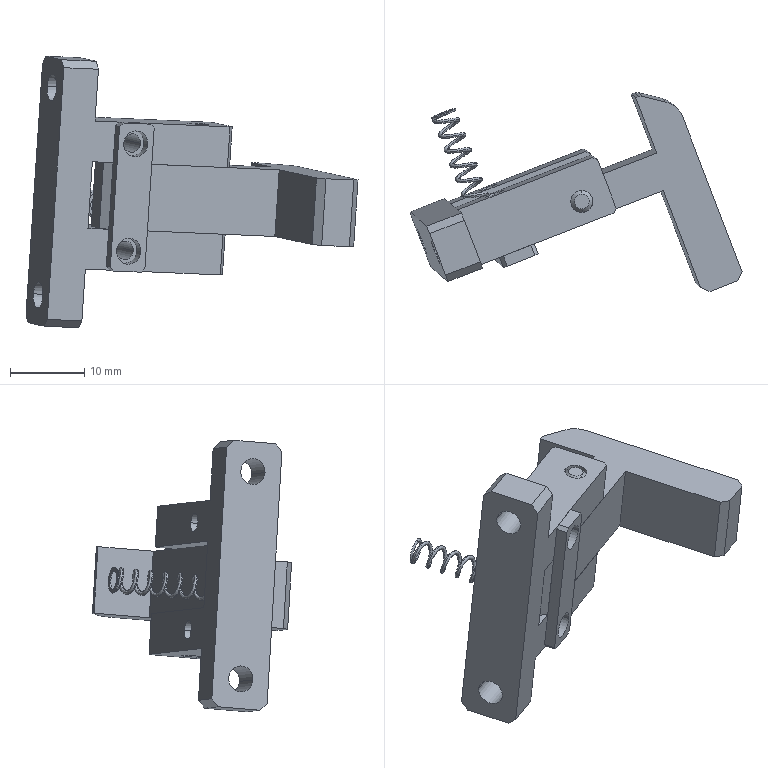Part | NX | features BREP 5 | 5 solids | 97 faces | box 44.679 x 26.792 x 36.53 mm | volume 5605 mm3 | plane 51 | cylinder 32 | cone 8 | torus 4 | spline 2 | commonest cylinder face diameters 2.5 x14 3 x8 3.5 x8 2 x1 6 x1